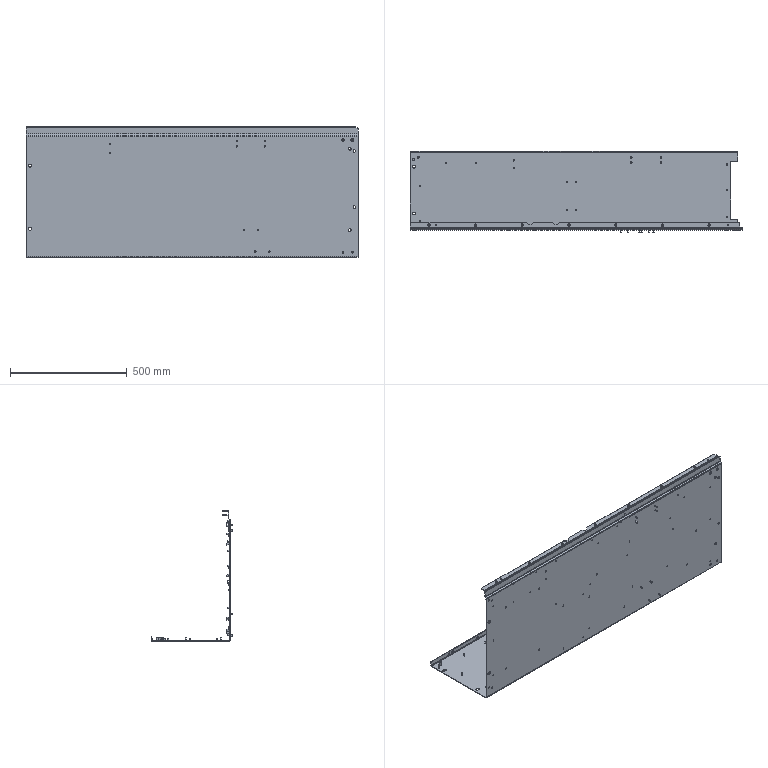Part | STEP file | 64741527 | 1 solid | 517 faces | box 1421 x 347.5 x 560 mm | volume 3305754 mm3 | cylinder 286 | plane 159 | torus 72 | commonest cylinder face diameters 6 x96 5 x39 8 x29 3.3 x28 8.3 x28 7.11 x22